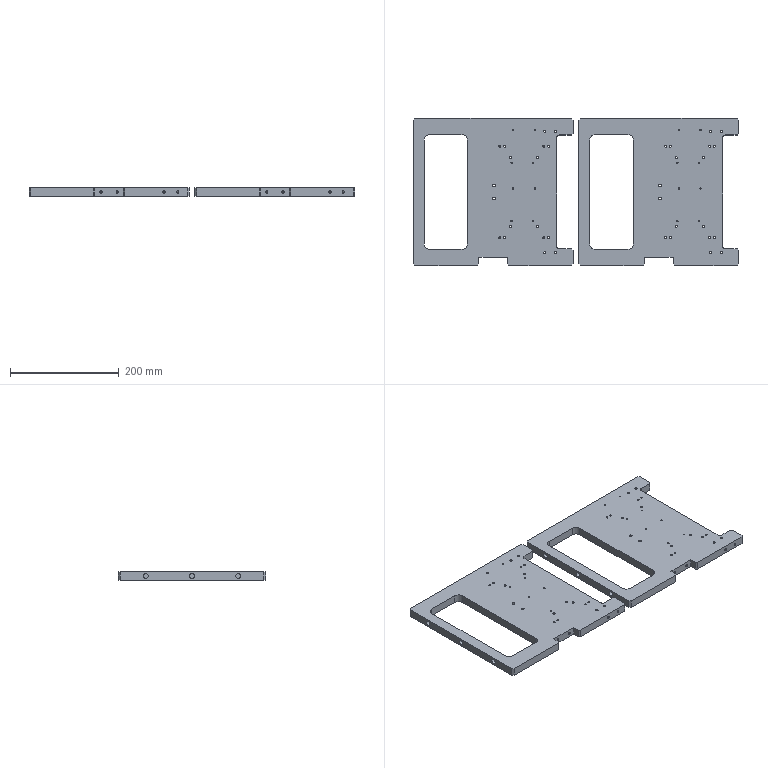Part | 2 solids | 146 faces | box 600 x 271 x 15 mm | volume 1659736 mm3 | cylinder 82 | plane 52 | cone 12 | commonest cylinder face diameters 4.2 x20 2.5 x16 3.3 x16 4 x8 20 x8 9 x6